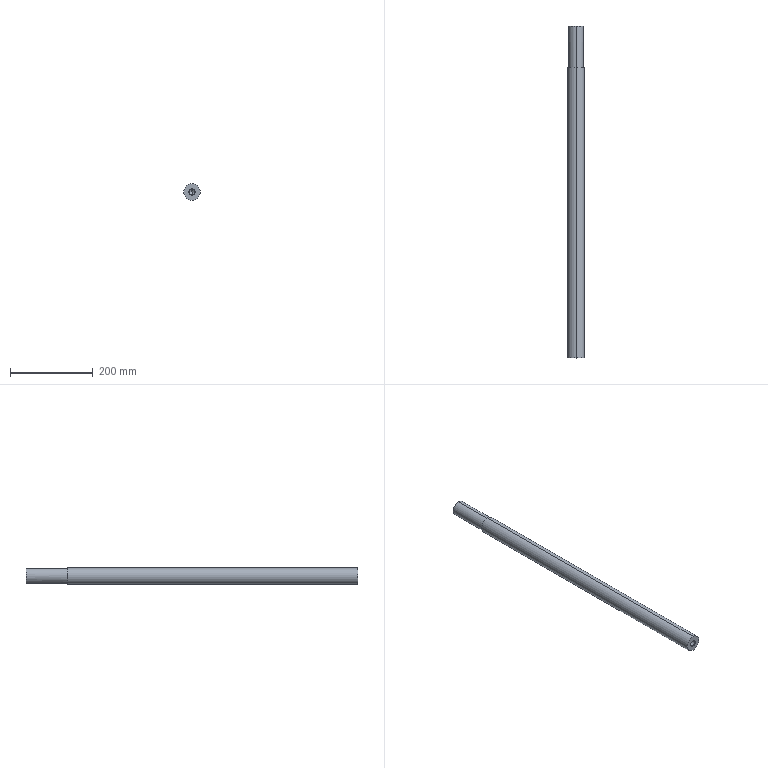Part | SolidWorks | features BaseBody 1 | 1 solid | 15 faces | box 40 x 800 x 40 mm | volume 974271 mm3 | cylinder 6 | cone 6 | plane 3 | commonest cylinder face diameters 14 x2 36 x2 40 x2
STEP:
#1=CARTESIAN_POINT('',(0.,700.,-20.));
#2=VERTEX_POINT('',#1);
#3=CARTESIAN_POINT('',(0.,700.,20.));
#4=VERTEX_POINT('',#3);
#5=CARTESIAN_POINT('',(0.,700.,0.));
#6=DIRECTION('',(0.,-1.,0.));
#7=DIRECTION('',(0.,0.,-1.));
#8=AXIS2_PLACEMENT_3D('',#5,#6,#7);
#9=CIRCLE('',#8,20.);
#10=EDGE_CURVE('',#2,#4,#9,.T.);
#11=ORIENTED_EDGE('',*,*,#10,.T.);
#12=CARTESIAN_POINT('',(0.,0.,20.));
#13=VERTEX_POINT('',#12);
#14=CARTESIAN_POINT('',(0.,700.,20.));
#15=DIRECTION('',(0.,-1.,0.));
#16=VECTOR('',#15,1000.);
#17=LINE('',#14,#16);
#18=EDGE_CURVE('',#4,#13,#17,.T.);
#19=ORIENTED_EDGE('',*,*,#18,.T.);
#20=CARTESIAN_POINT('',(0.,0.,-20.));
#21=VERTEX_POINT('',#20);
#22=CARTESIAN_POINT('',(0.,0.,0.));
#23=DIRECTION('',(0.,1.,0.));
#24=DIRECTION('',(0.,0.,-1.));
#25=AXIS2_PLACEMENT_3D('',#22,#23,#24);
#26=CIRCLE('',#25,20.);
#27=EDGE_CURVE('',#13,#21,#26,.T.);
#28=ORIENTED_EDGE('',*,*,#27,.T.);
#29=CARTESIAN_POINT('',(0.,700.,-20.));
#30=DIRECTION('',(0.,-1.,0.));
#31=VECTOR('',#30,1000.);
#32=LINE('',#29,#31);
#33=EDGE_CURVE('',#2,#21,#32,.T.);
#34=ORIENTED_EDGE('',*,*,#33,.F.);
#35=EDGE_LOOP('',(#11,#19,#28,#34));
#36=FACE_OUTER_BOUND('',#35,.T.);
#37=CARTESIAN_POINT('',(0.,700.,0.));
#38=DIRECTION('',(0.,-1.,0.));
#39=DIRECTION('',(0.,0.,-1.));
#40=AXIS2_PLACEMENT_3D('',#37,#38,#39);
#41=CYLINDRICAL_SURFACE('',#40,20.);
#42=ADVANCED_FACE('',(#36),#41,.T.);
#43=CARTESIAN_POINT('',(0.,0.5,7.));
#44=VERTEX_POINT('',#43);
#45=CARTESIAN_POINT('',(0.,0.5,-7.));
#46=VERTEX_POINT('',#45);
#47=CARTESIAN_POINT('',(0.,0.5,0.));
#48=DIRECTION('',(0.,-1.,0.));
#49=DIRECTION('',(0.,0.,-1.));
#50=AXIS2_PLACEMENT_3D('',#47,#48,#49);
#51=CIRCLE('',#50,7.);
#52=EDGE_CURVE('',#44,#46,#51,.T.);
#53=ORIENTED_EDGE('',*,*,#52,.F.);
#54=CARTESIAN_POINT('',(0.,0.,7.5));
#55=VERTEX_POINT('',#54);
#56=CARTESIAN_POINT('',(0.,0.,7.5));
#57=DIRECTION('',(0.,-0.7071,0.7071));
#58=VECTOR('',#57,1000.);
#59=LINE('',#56,#58);
#60=EDGE_CURVE('',#44,#55,#59,.T.);
#61=ORIENTED_EDGE('',*,*,#60,.T.);
#62=CARTESIAN_POINT('',(0.,0.,-7.5));
#63=VERTEX_POINT('',#62);
#64=CARTESIAN_POINT('',(0.,0.,0.));
#65=DIRECTION('',(0.,-1.,0.));
#66=DIRECTION('',(0.,0.,-1.));
#67=AXIS2_PLACEMENT_3D('',#64,#65,#66);
#68=CIRCLE('',#67,7.5);
#69=EDGE_CURVE('',#55,#63,#68,.T.);
#70=ORIENTED_EDGE('',*,*,#69,.T.);
#71=CARTESIAN_POINT('',(0.,0.,-7.5));
#72=DIRECTION('',(0.,-0.7071,-0.7071));
#73=VECTOR('',#72,1000.);
#74=LINE('',#71,#73);
#75=EDGE_CURVE('',#46,#63,#74,.T.);
#76=ORIENTED_EDGE('',*,*,#75,.F.);
#77=EDGE_LOOP('',(#53,#61,#70,#76));
#78=FACE_OUTER_BOUND('',#77,.T.);
#79=CARTESIAN_POINT('',(0.,0.,0.));
#80=DIRECTION('',(0.,-1.,0.));
#81=DIRECTION('',(0.,0.,-1.));
#82=AXIS2_PLACEMENT_3D('',#79,#80,#81);
#83=CONICAL_SURFACE('',#82,7.5,0.7854);
#84=ADVANCED_FACE('',(#78),#83,.F.);
#85=CARTESIAN_POINT('',(18.,799.5,0.));
#86=VERTEX_POINT('',#85);
#87=CARTESIAN_POINT('',(0.,799.5,18.));
#88=VERTEX_POINT('',#87);
#89=CARTESIAN_POINT('',(0.,799.5,0.));
#90=DIRECTION('',(0.,-1.,0.));
#91=DIRECTION('',(0.,0.,-1.));
#92=AXIS2_PLACEMENT_3D('',#89,#90,#91);
#93=CIRCLE('',#92,18.);
#94=EDGE_CURVE('',#86,#88,#93,.T.);
#95=ORIENTED_EDGE('',*,*,#94,.T.);
#96=CARTESIAN_POINT('',(0.,700.,18.));
#97=VERTEX_POINT('',#96);
#98=CARTESIAN_POINT('',(0.,800.,18.));
#99=DIRECTION('',(0.,-1.,0.));
#100=VECTOR('',#99,1000.);
#101=LINE('',#98,#100);
#102=EDGE_CURVE('',#88,#97,#101,.T.);
#103=ORIENTED_EDGE('',*,*,#102,.T.);
#104=CARTESIAN_POINT('',(0.,700.,-18.));
#105=VERTEX_POINT('',#104);
#106=CARTESIAN_POINT('',(0.,700.,0.));
#107=DIRECTION('',(0.,-1.,0.));
#108=DIRECTION('',(0.,0.,-1.));
#109=AXIS2_PLACEMENT_3D('',#106,#107,#108);
#110=CIRCLE('',#109,18.);
#111=EDGE_CURVE('',#105,#97,#110,.T.);
#112=ORIENTED_EDGE('',*,*,#111,.F.);
#113=CARTESIAN_POINT('',(0.,799.5,-18.));
#114=VERTEX_POINT('',#113);
#115=CARTESIAN_POINT('',(0.,800.,-18.));
#116=DIRECTION('',(0.,-1.,0.));
#117=VECTOR('',#116,1000.);
#118=LINE('',#115,#117);
#119=EDGE_CURVE('',#114,#105,#118,.T.);
#120=ORIENTED_EDGE('',*,*,#119,.F.);
#121=CARTESIAN_POINT('',(0.,799.5,0.));
#122=DIRECTION('',(0.,-1.,0.));
#123=DIRECTION('',(0.,0.,-1.));
#124=AXIS2_PLACEMENT_3D('',#121,#122,#123);
#125=CIRCLE('',#124,18.);
#126=EDGE_CURVE('',#114,#86,#125,.T.);
#127=ORIENTED_EDGE('',*,*,#126,.T.);
#128=EDGE_LOOP('',(#95,#103,#112,#120,#127));
#129=FACE_OUTER_BOUND('',#128,.T.);
#130=CARTESIAN_POINT('',(0.,800.,0.));
#131=DIRECTION('',(0.,-1.,0.));
#132=DIRECTION('',(0.,0.,-1.));
#133=AXIS2_PLACEMENT_3D('',#130,#131,#132);
#134=CYLINDRICAL_SURFACE('',#133,18.);
#135=ADVANCED_FACE('',(#129),#134,.T.);
#136=CARTESIAN_POINT('',(0.,45.,7.));
#137=VERTEX_POINT('',#136);
#138=CARTESIAN_POINT('',(0.,45.,-7.));
#139=VERTEX_POINT('',#138);
#140=CARTESIAN_POINT('',(0.,45.,0.));
#141=DIRECTION('',(0.,-1.,0.));
#142=DIRECTION('',(0.,0.,-1.));
#143=AXIS2_PLACEMENT_3D('',#140,#141,#142);
#144=CIRCLE('',#143,7.);
#145=EDGE_CURVE('',#137,#139,#144,.T.);
#146=ORIENTED_EDGE('',*,*,#145,.F.);
#147=CARTESIAN_POINT('',(0.,0.,7.));
#148=DIRECTION('',(0.,-1.,0.));
#149=VECTOR('',#148,1000.);
#150=LINE('',#147,#149);
#151=EDGE_CURVE('',#137,#44,#150,.T.);
#152=ORIENTED_EDGE('',*,*,#151,.T.);
#153=ORIENTED_EDGE('',*,*,#52,.T.);
#154=CARTESIAN_POINT('',(0.,0.,-7.));
#155=DIRECTION('',(0.,-1.,0.));
#156=VECTOR('',#155,1000.);
#157=LINE('',#154,#156);
#158=EDGE_CURVE('',#139,#46,#157,.T.);
#159=ORIENTED_EDGE('',*,*,#158,.F.);
#160=EDGE_LOOP('',(#146,#152,#153,#159));
#161=FACE_OUTER_BOUND('',#160,.T.);
#162=CARTESIAN_POINT('',(0.,0.,0.));
#163=DIRECTION('',(0.,-1.,0.));
#164=DIRECTION('',(0.,0.,-1.));
#165=AXIS2_PLACEMENT_3D('',#162,#163,#164);
#166=CYLINDRICAL_SURFACE('',#165,7.);
#167=ADVANCED_FACE('',(#161),#166,.F.);
#168=CARTESIAN_POINT('',(17.5,800.,0.));
#169=VERTEX_POINT('',#168);
#170=CARTESIAN_POINT('',(-17.5,800.,0.));
#171=VERTEX_POINT('',#170);
#172=CARTESIAN_POINT('',(0.,800.,0.));
#173=DIRECTION('',(0.,-1.,0.));
#174=DIRECTION('',(1.,0.,0.));
#175=AXIS2_PLACEMENT_3D('',#172,#173,#174);
#176=CIRCLE('',#175,17.5);
#177=EDGE_CURVE('',#169,#171,#176,.T.);
#178=ORIENTED_EDGE('',*,*,#177,.T.);
#179=CARTESIAN_POINT('',(-18.,799.5,0.));
#180=VERTEX_POINT('',#179);
#181=CARTESIAN_POINT('',(-18.,799.5,0.));
#182=DIRECTION('',(-0.7071,-0.7071,0.));
#183=VECTOR('',#182,1000.);
#184=LINE('',#181,#183);
#185=EDGE_CURVE('',#171,#180,#184,.T.);
#186=ORIENTED_EDGE('',*,*,#185,.T.);
#187=CARTESIAN_POINT('',(0.,799.5,0.));
#188=DIRECTION('',(0.,-1.,0.));
#189=DIRECTION('',(0.,0.,-1.));
#190=AXIS2_PLACEMENT_3D('',#187,#188,#189);
#191=CIRCLE('',#190,18.);
#192=EDGE_CURVE('',#88,#180,#191,.T.);
#193=ORIENTED_EDGE('',*,*,#192,.F.);
#194=ORIENTED_EDGE('',*,*,#94,.F.);
#195=CARTESIAN_POINT('',(18.,799.5,0.));
#196=DIRECTION('',(0.7071,-0.7071,0.));
#197=VECTOR('',#196,1000.);
#198=LINE('',#195,#197);
#199=EDGE_CURVE('',#169,#86,#198,.T.);
#200=ORIENTED_EDGE('',*,*,#199,.F.);
#201=EDGE_LOOP('',(#178,#186,#193,#194,#200));
#202=FACE_OUTER_BOUND('',#201,.T.);
#203=CARTESIAN_POINT('',(0.,799.5,0.));
#204=DIRECTION('',(0.,-1.,0.));
#205=DIRECTION('',(1.,0.,0.));
#206=AXIS2_PLACEMENT_3D('',#203,#204,#205);
#207=CONICAL_SURFACE('',#206,18.,0.7854);
#208=ADVANCED_FACE('',(#202),#207,.T.);
#209=CARTESIAN_POINT('',(0.,49.206,0.));
#210=VERTEX_POINT('',#209);
#211=CARTESIAN_POINT('',(0.,45.,-7.));
#212=DIRECTION('',(0.,-0.515,-0.8572));
#213=VECTOR('',#212,1000.);
#214=LINE('',#211,#213);
#215=EDGE_CURVE('',#210,#139,#214,.T.);
#216=ORIENTED_EDGE('',*,*,#215,.F.);
#217=CARTESIAN_POINT('',(0.,45.,7.));
#218=DIRECTION('',(0.,-0.515,0.8572));
#219=VECTOR('',#218,1000.);
#220=LINE('',#217,#219);
#221=EDGE_CURVE('',#210,#137,#220,.T.);
#222=ORIENTED_EDGE('',*,*,#221,.T.);
#223=ORIENTED_EDGE('',*,*,#145,.T.);
#224=EDGE_LOOP('',(#216,#222,#223));
#225=FACE_OUTER_BOUND('',#224,.T.);
#226=CARTESIAN_POINT('',(0.,45.,0.));
#227=DIRECTION('',(0.,-1.,0.));
#228=DIRECTION('',(0.,0.,-1.));
#229=AXIS2_PLACEMENT_3D('',#226,#227,#228);
#230=CONICAL_SURFACE('',#229,7.,1.03);
#231=ADVANCED_FACE('',(#225),#230,.F.);
#232=ORIENTED_EDGE('',*,*,#18,.F.);
#233=CARTESIAN_POINT('',(0.,700.,0.));
#234=DIRECTION('',(0.,-1.,0.));
#235=DIRECTION('',(0.,0.,-1.));
#236=AXIS2_PLACEMENT_3D('',#233,#234,#235);
#237=CIRCLE('',#236,20.);
#238=EDGE_CURVE('',#4,#2,#237,.T.);
#239=ORIENTED_EDGE('',*,*,#238,.T.);
#240=ORIENTED_EDGE('',*,*,#33,.T.);
#241=CARTESIAN_POINT('',(0.,0.,0.));
#242=DIRECTION('',(0.,1.,0.));
#243=DIRECTION('',(0.,0.,-1.));
#244=AXIS2_PLACEMENT_3D('',#241,#242,#243);
#245=CIRCLE('',#244,20.);
#246=EDGE_CURVE('',#21,#13,#245,.T.);
#247=ORIENTED_EDGE('',*,*,#246,.T.);
#248=EDGE_LOOP('',(#232,#239,#240,#247));
#249=FACE_OUTER_BOUND('',#248,.T.);
#250=CARTESIAN_POINT('',(0.,700.,0.));
#251=DIRECTION('',(0.,-1.,0.));
#252=DIRECTION('',(0.,0.,-1.));
#253=AXIS2_PLACEMENT_3D('',#250,#251,#252);
#254=CYLINDRICAL_SURFACE('',#253,20.);
#255=ADVANCED_FACE('',(#249),#254,.T.);
#256=ORIENTED_EDGE('',*,*,#246,.F.);
#257=ORIENTED_EDGE('',*,*,#27,.F.);
#258=EDGE_LOOP('',(#256,#257));
#259=FACE_OUTER_BOUND('',#258,.T.);
#260=CARTESIAN_POINT('',(0.,0.,0.));
#261=DIRECTION('',(0.,-1.,0.));
#262=DIRECTION('',(0.,0.,-1.));
#263=AXIS2_PLACEMENT_3D('',#260,#261,#262);
#264=CIRCLE('',#263,7.5);
#265=EDGE_CURVE('',#63,#55,#264,.T.);
#266=ORIENTED_EDGE('',*,*,#265,.F.);
#267=ORIENTED_EDGE('',*,*,#69,.F.);
#268=EDGE_LOOP('',(#266,#267));
#269=FACE_BOUND('',#268,.T.);
#270=CARTESIAN_POINT('',(0.,0.,0.));
#271=DIRECTION('',(0.,1.,0.));
#272=DIRECTION('',(0.,0.,1.));
#273=AXIS2_PLACEMENT_3D('',#270,#271,#272);
#274=PLANE('',#273);
#275=ADVANCED_FACE('',(#259,#269),#274,.F.);
#276=ORIENTED_EDGE('',*,*,#10,.F.);
#277=ORIENTED_EDGE('',*,*,#238,.F.);
#278=EDGE_LOOP('',(#276,#277));
#279=FACE_OUTER_BOUND('',#278,.T.);
#280=ORIENTED_EDGE('',*,*,#111,.T.);
#281=CARTESIAN_POINT('',(0.,700.,0.));
#282=DIRECTION('',(0.,-1.,0.));
#283=DIRECTION('',(0.,0.,-1.));
#284=AXIS2_PLACEMENT_3D('',#281,#282,#283);
#285=CIRCLE('',#284,18.);
#286=EDGE_CURVE('',#97,#105,#285,.T.);
#287=ORIENTED_EDGE('',*,*,#286,.T.);
#288=EDGE_LOOP('',(#280,#287));
#289=FACE_BOUND('',#288,.T.);
#290=CARTESIAN_POINT('',(0.,700.,0.));
#291=DIRECTION('',(0.,1.,0.));
#292=DIRECTION('',(0.,0.,1.));
#293=AXIS2_PLACEMENT_3D('',#290,#291,#292);
#294=PLANE('',#293);
#295=ADVANCED_FACE('',(#279,#289),#294,.T.);
#296=ORIENTED_EDGE('',*,*,#60,.F.);
#297=CARTESIAN_POINT('',(0.,0.5,0.));
#298=DIRECTION('',(0.,-1.,0.));
#299=DIRECTION('',(0.,0.,-1.));
#300=AXIS2_PLACEMENT_3D('',#297,#298,#299);
#301=CIRCLE('',#300,7.);
#302=EDGE_CURVE('',#46,#44,#301,.T.);
#303=ORIENTED_EDGE('',*,*,#302,.F.);
#304=ORIENTED_EDGE('',*,*,#75,.T.);
#305=ORIENTED_EDGE('',*,*,#265,.T.);
#306=EDGE_LOOP('',(#296,#303,#304,#305));
#307=FACE_OUTER_BOUND('',#306,.T.);
#308=CARTESIAN_POINT('',(0.,0.,0.));
#309=DIRECTION('',(0.,-1.,0.));
#310=DIRECTION('',(0.,0.,-1.));
#311=AXIS2_PLACEMENT_3D('',#308,#309,#310);
#312=CONICAL_SURFACE('',#311,7.5,0.7854);
#313=ADVANCED_FACE('',(#307),#312,.F.);
#314=ORIENTED_EDGE('',*,*,#102,.F.);
#315=ORIENTED_EDGE('',*,*,#192,.T.);
#316=CARTESIAN_POINT('',(0.,799.5,0.));
#317=DIRECTION('',(0.,-1.,0.));
#318=DIRECTION('',(0.,0.,-1.));
#319=AXIS2_PLACEMENT_3D('',#316,#317,#318);
#320=CIRCLE('',#319,18.);
#321=EDGE_CURVE('',#180,#114,#320,.T.);
#322=ORIENTED_EDGE('',*,*,#321,.T.);
#323=ORIENTED_EDGE('',*,*,#119,.T.);
#324=ORIENTED_EDGE('',*,*,#286,.F.);
#325=EDGE_LOOP('',(#314,#315,#322,#323,#324));
#326=FACE_OUTER_BOUND('',#325,.T.);
#327=CARTESIAN_POINT('',(0.,800.,0.));
#328=DIRECTION('',(0.,-1.,0.));
#329=DIRECTION('',(0.,0.,-1.));
#330=AXIS2_PLACEMENT_3D('',#327,#328,#329);
#331=CYLINDRICAL_SURFACE('',#330,18.);
#332=ADVANCED_FACE('',(#326),#331,.T.);
#333=ORIENTED_EDGE('',*,*,#151,.F.);
#334=CARTESIAN_POINT('',(0.,45.,0.));
#335=DIRECTION('',(0.,-1.,0.));
#336=DIRECTION('',(0.,0.,-1.));
#337=AXIS2_PLACEMENT_3D('',#334,#335,#336);
#338=CIRCLE('',#337,7.);
#339=EDGE_CURVE('',#139,#137,#338,.T.);
#340=ORIENTED_EDGE('',*,*,#339,.F.);
#341=ORIENTED_EDGE('',*,*,#158,.T.);
#342=ORIENTED_EDGE('',*,*,#302,.T.);
#343=EDGE_LOOP('',(#333,#340,#341,#342));
#344=FACE_OUTER_BOUND('',#343,.T.);
#345=CARTESIAN_POINT('',(0.,0.,0.));
#346=DIRECTION('',(0.,-1.,0.));
#347=DIRECTION('',(0.,0.,-1.));
#348=AXIS2_PLACEMENT_3D('',#345,#346,#347);
#349=CYLINDRICAL_SURFACE('',#348,7.);
#350=ADVANCED_FACE('',(#344),#349,.F.);
#351=ORIENTED_EDGE('',*,*,#185,.F.);
#352=CARTESIAN_POINT('',(0.,800.,0.));
#353=DIRECTION('',(0.,-1.,0.));
#354=DIRECTION('',(1.,0.,0.));
#355=AXIS2_PLACEMENT_3D('',#352,#353,#354);
#356=CIRCLE('',#355,17.5);
#357=EDGE_CURVE('',#171,#169,#356,.T.);
#358=ORIENTED_EDGE('',*,*,#357,.T.);
#359=ORIENTED_EDGE('',*,*,#199,.T.);
#360=ORIENTED_EDGE('',*,*,#126,.F.);
#361=ORIENTED_EDGE('',*,*,#321,.F.);
#362=EDGE_LOOP('',(#351,#358,#359,#360,#361));
#363=FACE_OUTER_BOUND('',#362,.T.);
#364=CARTESIAN_POINT('',(0.,799.5,0.));
#365=DIRECTION('',(0.,-1.,0.));
#366=DIRECTION('',(1.,0.,0.));
#367=AXIS2_PLACEMENT_3D('',#364,#365,#366);
#368=CONICAL_SURFACE('',#367,18.,0.7854);
#369=ADVANCED_FACE('',(#363),#368,.T.);
#370=ORIENTED_EDGE('',*,*,#221,.F.);
#371=ORIENTED_EDGE('',*,*,#215,.T.);
#372=ORIENTED_EDGE('',*,*,#339,.T.);
#373=EDGE_LOOP('',(#370,#371,#372));
#374=FACE_OUTER_BOUND('',#373,.T.);
#375=CARTESIAN_POINT('',(0.,45.,0.));
#376=DIRECTION('',(0.,-1.,0.));
#377=DIRECTION('',(0.,0.,-1.));
#378=AXIS2_PLACEMENT_3D('',#375,#376,#377);
#379=CONICAL_SURFACE('',#378,7.,1.03);
#380=ADVANCED_FACE('',(#374),#379,.F.);
#381=ORIENTED_EDGE('',*,*,#177,.F.);
#382=ORIENTED_EDGE('',*,*,#357,.F.);
#383=EDGE_LOOP('',(#381,#382));
#384=FACE_OUTER_BOUND('',#383,.T.);
#385=CARTESIAN_POINT('',(0.,800.,0.));
#386=DIRECTION('',(0.,1.,0.));
#387=DIRECTION('',(0.,0.,1.));
#388=AXIS2_PLACEMENT_3D('',#385,#386,#387);
#389=PLANE('',#388);
#390=ADVANCED_FACE('',(#384),#389,.T.);
#391=CLOSED_SHELL('',(#42,#84,#135,#167,#208,#231,#255,#275,#295,#313,#332,#350,#369,#380,#390));
#392=MANIFOLD_SOLID_BREP('',#391);
#393=CARTESIAN_POINT('',(0.,0.,0.));
#394=DIRECTION('',(0.,0.,1.));
#395=DIRECTION('',(1.,0.,0.));
#396=AXIS2_PLACEMENT_3D('',#393,#394,#395);
#397=(LENGTH_UNIT()NAMED_UNIT(*)SI_UNIT(.MILLI.,.METRE.));
#398=UNCERTAINTY_MEASURE_WITH_UNIT(LENGTH_MEASURE(0.00001),#397,'','');
#399=(NAMED_UNIT(*)PLANE_ANGLE_UNIT()SI_UNIT($,.RADIAN.));
#400=(NAMED_UNIT(*)SI_UNIT($,.STERADIAN.)SOLID_ANGLE_UNIT());
#401=(GEOMETRIC_REPRESENTATION_CONTEXT(3)GLOBAL_UNCERTAINTY_ASSIGNED_CONTEXT((#398))GLOBAL_UNIT_ASSIGNED_CONTEXT((#397,#399,#400))REPRESENTATION_CONTEXT('',''));
#402=ADVANCED_BREP_SHAPE_REPRESENTATION('',(#392,#396),#401);